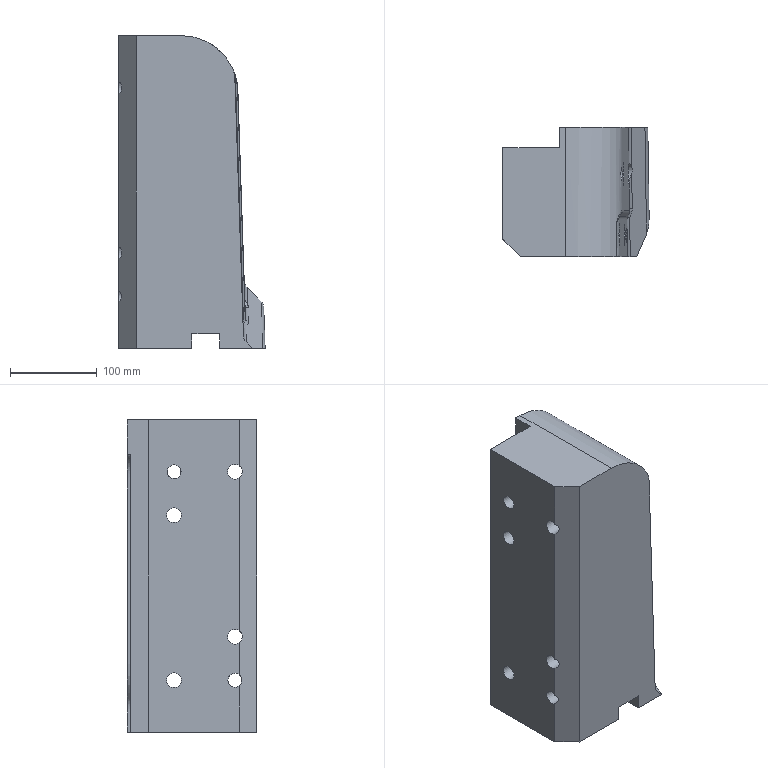Part | NX | features solid 2 | 1 solid | 50 faces | box 168.35 x 148.71 x 360.008 mm | volume 6398414 mm3 | plane 20 | cylinder 20 | spline 9 | sphere 1 | commonest cylinder face diameters 20 x5 16 x4 17 x4 26 x4 16.056 x1 60 x1